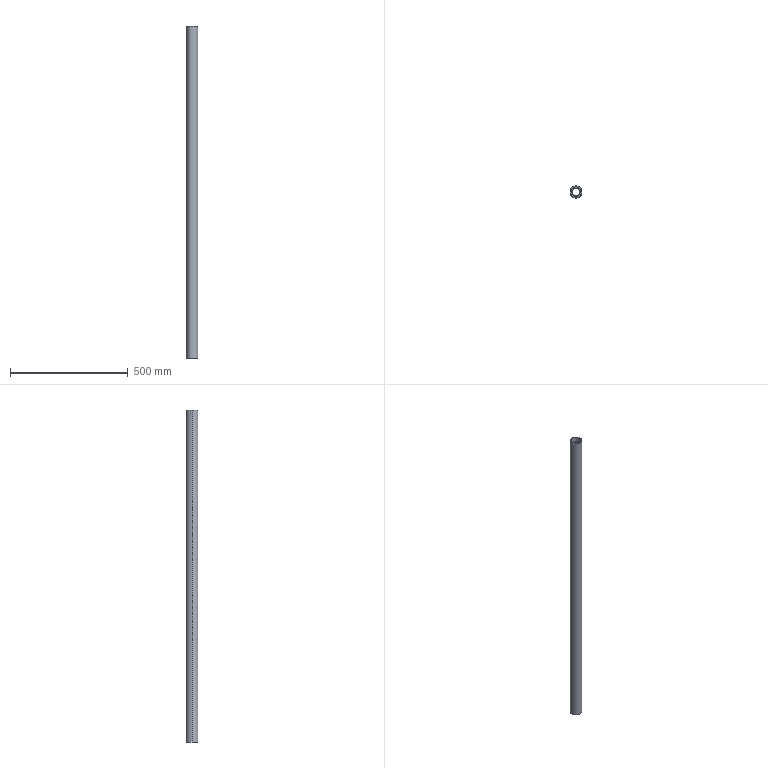Part | STEP file | 1 solid | 12 faces | box 50 x 50 x 1410 mm | volume 1744715 mm3 | cylinder 8 | plane 4 | commonest cylinder face diameters 42 x4 30 x2 50 x2
STEP:
#1=CARTESIAN_POINT('',(0.,0.,0.));
#2=DIRECTION('',(0.,0.,1.));
#3=DIRECTION('',(1.,0.,0.));
#4=AXIS2_PLACEMENT_3D('',#1,#2,#3);
#5=CARTESIAN_POINT('',(-21.,0.,-665.));
#6=VERTEX_POINT('',#5);
#7=CARTESIAN_POINT('',(-21.,0.,-685.));
#8=VERTEX_POINT('',#7);
#9=CARTESIAN_POINT('',(-21.,0.,-705.));
#10=DIRECTION('',(0.,0.,-1.));
#11=VECTOR('',#10,1.);
#12=LINE('',#9,#11);
#13=CARTESIAN_POINT('',(0.,0.,-705.));
#14=DIRECTION('',(0.,0.,-1.));
#15=DIRECTION('',(-1.,0.,0.));
#16=AXIS2_PLACEMENT_3D('',#13,#14,#15);
#17=CYLINDRICAL_SURFACE('',#16,21.);
#18=CARTESIAN_POINT('',(6.283,0.));
#19=DIRECTION('',(0.,1.));
#20=VECTOR('',#19,1.);
#21=LINE('',#18,#20);
#22=(GEOMETRIC_REPRESENTATION_CONTEXT(2)PARAMETRIC_REPRESENTATION_CONTEXT()REPRESENTATION_CONTEXT('',''));
#23=DEFINITIONAL_REPRESENTATION('',(#21),#22);
#24=PCURVE('',#17,#23);
#25=CARTESIAN_POINT('',(0.,0.,-705.));
#26=DIRECTION('',(0.,0.,-1.));
#27=DIRECTION('',(-1.,0.,0.));
#28=AXIS2_PLACEMENT_3D('',#25,#26,#27);
#29=CYLINDRICAL_SURFACE('',#28,21.);
#30=CARTESIAN_POINT('',(0.,0.));
#31=DIRECTION('',(0.,1.));
#32=VECTOR('',#31,1.);
#33=LINE('',#30,#32);
#34=(GEOMETRIC_REPRESENTATION_CONTEXT(2)PARAMETRIC_REPRESENTATION_CONTEXT()REPRESENTATION_CONTEXT('',''));
#35=DEFINITIONAL_REPRESENTATION('',(#33),#34);
#36=PCURVE('',#29,#35);
#37=SURFACE_CURVE('',#12,(#24,#36),.PCURVE_S1.);
#38=EDGE_CURVE('',#6,#8,#37,.T.);
#39=ORIENTED_EDGE('',*,*,#38,.T.);
#40=CARTESIAN_POINT('',(21.,0.,-685.));
#41=VERTEX_POINT('',#40);
#42=CARTESIAN_POINT('',(0.,0.,-685.));
#43=DIRECTION('',(0.,0.,1.));
#44=DIRECTION('',(1.,0.,0.));
#45=AXIS2_PLACEMENT_3D('',#42,#43,#44);
#46=CIRCLE('',#45,21.);
#47=CARTESIAN_POINT('',(9.425,-20.));
#48=DIRECTION('',(-1.,0.));
#49=VECTOR('',#48,1.);
#50=LINE('',#47,#49);
#51=(GEOMETRIC_REPRESENTATION_CONTEXT(2)PARAMETRIC_REPRESENTATION_CONTEXT()REPRESENTATION_CONTEXT('',''));
#52=DEFINITIONAL_REPRESENTATION('',(#50),#51);
#53=PCURVE('',#17,#52);
#54=CARTESIAN_POINT('',(0.,0.,-685.));
#55=DIRECTION('',(0.,0.,1.));
#56=DIRECTION('',(1.,0.,0.));
#57=AXIS2_PLACEMENT_3D('',#54,#55,#56);
#58=PLANE('',#57);
#59=CARTESIAN_POINT('',(0.,0.));
#60=DIRECTION('',(1.,0.));
#61=AXIS2_PLACEMENT_2D('',#59,#60);
#62=CIRCLE('',#61,21.);
#63=(GEOMETRIC_REPRESENTATION_CONTEXT(2)PARAMETRIC_REPRESENTATION_CONTEXT()REPRESENTATION_CONTEXT('',''));
#64=DEFINITIONAL_REPRESENTATION('',(#62),#63);
#65=PCURVE('',#58,#64);
#66=SURFACE_CURVE('',#46,(#53,#65),.PCURVE_S1.);
#67=EDGE_CURVE('',#8,#41,#66,.T.);
#68=ORIENTED_EDGE('',*,*,#67,.T.);
#69=CARTESIAN_POINT('',(21.,0.,-665.));
#70=VERTEX_POINT('',#69);
#71=CARTESIAN_POINT('',(21.,0.,-705.));
#72=DIRECTION('',(0.,0.,-1.));
#73=VECTOR('',#72,1.);
#74=LINE('',#71,#73);
#75=CARTESIAN_POINT('',(3.142,0.));
#76=DIRECTION('',(0.,1.));
#77=VECTOR('',#76,1.);
#78=LINE('',#75,#77);
#79=(GEOMETRIC_REPRESENTATION_CONTEXT(2)PARAMETRIC_REPRESENTATION_CONTEXT()REPRESENTATION_CONTEXT('',''));
#80=DEFINITIONAL_REPRESENTATION('',(#78),#79);
#81=PCURVE('',#17,#80);
#82=CARTESIAN_POINT('',(3.142,0.));
#83=DIRECTION('',(0.,1.));
#84=VECTOR('',#83,1.);
#85=LINE('',#82,#84);
#86=(GEOMETRIC_REPRESENTATION_CONTEXT(2)PARAMETRIC_REPRESENTATION_CONTEXT()REPRESENTATION_CONTEXT('',''));
#87=DEFINITIONAL_REPRESENTATION('',(#85),#86);
#88=PCURVE('',#29,#87);
#89=SURFACE_CURVE('',#74,(#81,#88),.PCURVE_S1.);
#90=EDGE_CURVE('',#70,#41,#89,.T.);
#91=ORIENTED_EDGE('',*,*,#90,.F.);
#92=CARTESIAN_POINT('',(0.,0.,-665.));
#93=DIRECTION('',(0.,0.,1.));
#94=DIRECTION('',(-1.,0.,0.));
#95=AXIS2_PLACEMENT_3D('',#92,#93,#94);
#96=CIRCLE('',#95,21.);
#97=CARTESIAN_POINT('',(6.283,-40.));
#98=DIRECTION('',(-1.,0.));
#99=VECTOR('',#98,1.);
#100=LINE('',#97,#99);
#101=(GEOMETRIC_REPRESENTATION_CONTEXT(2)PARAMETRIC_REPRESENTATION_CONTEXT()REPRESENTATION_CONTEXT('',''));
#102=DEFINITIONAL_REPRESENTATION('',(#100),#101);
#103=PCURVE('',#17,#102);
#104=CARTESIAN_POINT('',(0.,0.,-665.));
#105=DIRECTION('',(0.,0.,-1.));
#106=DIRECTION('',(1.,0.,0.));
#107=AXIS2_PLACEMENT_3D('',#104,#105,#106);
#108=PLANE('',#107);
#109=CARTESIAN_POINT('',(-21.,0.));
#110=CARTESIAN_POINT('',(-21.,36.373));
#111=CARTESIAN_POINT('',(10.5,18.187));
#112=CARTESIAN_POINT('',(42.,0.));
#113=CARTESIAN_POINT('',(10.5,-18.187));
#114=CARTESIAN_POINT('',(-21.,-36.373));
#115=CARTESIAN_POINT('',(-21.,0.));
#116=(BOUNDED_CURVE()B_SPLINE_CURVE(2,(#109,#110,#111,#112,#113,#114,#115),.UNSPECIFIED.,.T.,.F.)B_SPLINE_CURVE_WITH_KNOTS((1,2,2,2,2,1),(-2.094,0.,2.094,4.189,6.283,8.378),.UNSPECIFIED.)CURVE()GEOMETRIC_REPRESENTATION_ITEM()RATIONAL_B_SPLINE_CURVE((1.,0.5,1.,0.5,1.,0.5,1.))REPRESENTATION_ITEM(''));
#117=(GEOMETRIC_REPRESENTATION_CONTEXT(2)PARAMETRIC_REPRESENTATION_CONTEXT()REPRESENTATION_CONTEXT('',''));
#118=DEFINITIONAL_REPRESENTATION('',(#116),#117);
#119=PCURVE('',#108,#118);
#120=SURFACE_CURVE('',#96,(#103,#119),.PCURVE_S1.);
#121=EDGE_CURVE('',#6,#70,#120,.T.);
#122=ORIENTED_EDGE('',*,*,#121,.F.);
#123=EDGE_LOOP('',(#39,#68,#91,#122));
#124=FACE_BOUND('',#123,.F.);
#125=ADVANCED_FACE('',(#124),#17,.F.);
#126=CARTESIAN_POINT('',(21.,0.,705.));
#127=VERTEX_POINT('',#126);
#128=CARTESIAN_POINT('',(21.,0.,725.));
#129=VERTEX_POINT('',#128);
#130=CARTESIAN_POINT('',(21.,0.,705.));
#131=DIRECTION('',(0.,0.,1.));
#132=VECTOR('',#131,1.);
#133=LINE('',#130,#132);
#134=CARTESIAN_POINT('',(0.,0.,705.));
#135=DIRECTION('',(0.,0.,1.));
#136=DIRECTION('',(1.,0.,0.));
#137=AXIS2_PLACEMENT_3D('',#134,#135,#136);
#138=CYLINDRICAL_SURFACE('',#137,21.);
#139=CARTESIAN_POINT('',(6.283,0.));
#140=DIRECTION('',(0.,1.));
#141=VECTOR('',#140,1.);
#142=LINE('',#139,#141);
#143=(GEOMETRIC_REPRESENTATION_CONTEXT(2)PARAMETRIC_REPRESENTATION_CONTEXT()REPRESENTATION_CONTEXT('',''));
#144=DEFINITIONAL_REPRESENTATION('',(#142),#143);
#145=PCURVE('',#138,#144);
#146=CARTESIAN_POINT('',(0.,0.,705.));
#147=DIRECTION('',(0.,0.,1.));
#148=DIRECTION('',(1.,0.,0.));
#149=AXIS2_PLACEMENT_3D('',#146,#147,#148);
#150=CYLINDRICAL_SURFACE('',#149,21.);
#151=CARTESIAN_POINT('',(0.,0.));
#152=DIRECTION('',(0.,1.));
#153=VECTOR('',#152,1.);
#154=LINE('',#151,#153);
#155=(GEOMETRIC_REPRESENTATION_CONTEXT(2)PARAMETRIC_REPRESENTATION_CONTEXT()REPRESENTATION_CONTEXT('',''));
#156=DEFINITIONAL_REPRESENTATION('',(#154),#155);
#157=PCURVE('',#150,#156);
#158=SURFACE_CURVE('',#133,(#145,#157),.PCURVE_S1.);
#159=EDGE_CURVE('',#127,#129,#158,.T.);
#160=ORIENTED_EDGE('',*,*,#159,.T.);
#161=CARTESIAN_POINT('',(-21.,0.,725.));
#162=VERTEX_POINT('',#161);
#163=CARTESIAN_POINT('',(0.,0.,725.));
#164=DIRECTION('',(0.,0.,1.));
#165=DIRECTION('',(1.,0.,0.));
#166=AXIS2_PLACEMENT_3D('',#163,#164,#165);
#167=CIRCLE('',#166,21.);
#168=CARTESIAN_POINT('',(0.,20.));
#169=DIRECTION('',(1.,0.));
#170=VECTOR('',#169,1.);
#171=LINE('',#168,#170);
#172=(GEOMETRIC_REPRESENTATION_CONTEXT(2)PARAMETRIC_REPRESENTATION_CONTEXT()REPRESENTATION_CONTEXT('',''));
#173=DEFINITIONAL_REPRESENTATION('',(#171),#172);
#174=PCURVE('',#138,#173);
#175=CARTESIAN_POINT('',(0.,0.,725.));
#176=DIRECTION('',(0.,0.,1.));
#177=DIRECTION('',(1.,0.,0.));
#178=AXIS2_PLACEMENT_3D('',#175,#176,#177);
#179=PLANE('',#178);
#180=CARTESIAN_POINT('',(0.,0.));
#181=DIRECTION('',(1.,0.));
#182=AXIS2_PLACEMENT_2D('',#180,#181);
#183=CIRCLE('',#182,21.);
#184=(GEOMETRIC_REPRESENTATION_CONTEXT(2)PARAMETRIC_REPRESENTATION_CONTEXT()REPRESENTATION_CONTEXT('',''));
#185=DEFINITIONAL_REPRESENTATION('',(#183),#184);
#186=PCURVE('',#179,#185);
#187=SURFACE_CURVE('',#167,(#174,#186),.PCURVE_S1.);
#188=EDGE_CURVE('',#162,#129,#187,.T.);
#189=ORIENTED_EDGE('',*,*,#188,.F.);
#190=CARTESIAN_POINT('',(-21.,0.,705.));
#191=VERTEX_POINT('',#190);
#192=CARTESIAN_POINT('',(-21.,0.,705.));
#193=DIRECTION('',(0.,0.,1.));
#194=VECTOR('',#193,1.);
#195=LINE('',#192,#194);
#196=CARTESIAN_POINT('',(3.142,0.));
#197=DIRECTION('',(0.,1.));
#198=VECTOR('',#197,1.);
#199=LINE('',#196,#198);
#200=(GEOMETRIC_REPRESENTATION_CONTEXT(2)PARAMETRIC_REPRESENTATION_CONTEXT()REPRESENTATION_CONTEXT('',''));
#201=DEFINITIONAL_REPRESENTATION('',(#199),#200);
#202=PCURVE('',#138,#201);
#203=CARTESIAN_POINT('',(3.142,0.));
#204=DIRECTION('',(0.,1.));
#205=VECTOR('',#204,1.);
#206=LINE('',#203,#205);
#207=(GEOMETRIC_REPRESENTATION_CONTEXT(2)PARAMETRIC_REPRESENTATION_CONTEXT()REPRESENTATION_CONTEXT('',''));
#208=DEFINITIONAL_REPRESENTATION('',(#206),#207);
#209=PCURVE('',#150,#208);
#210=SURFACE_CURVE('',#195,(#202,#209),.PCURVE_S1.);
#211=EDGE_CURVE('',#191,#162,#210,.T.);
#212=ORIENTED_EDGE('',*,*,#211,.F.);
#213=CARTESIAN_POINT('',(0.,0.,705.));
#214=DIRECTION('',(0.,0.,1.));
#215=DIRECTION('',(1.,0.,0.));
#216=AXIS2_PLACEMENT_3D('',#213,#214,#215);
#217=CIRCLE('',#216,21.);
#218=CARTESIAN_POINT('',(0.,0.));
#219=DIRECTION('',(1.,0.));
#220=VECTOR('',#219,1.);
#221=LINE('',#218,#220);
#222=(GEOMETRIC_REPRESENTATION_CONTEXT(2)PARAMETRIC_REPRESENTATION_CONTEXT()REPRESENTATION_CONTEXT('',''));
#223=DEFINITIONAL_REPRESENTATION('',(#221),#222);
#224=PCURVE('',#138,#223);
#225=CARTESIAN_POINT('',(0.,0.,705.));
#226=DIRECTION('',(0.,0.,1.));
#227=DIRECTION('',(1.,0.,0.));
#228=AXIS2_PLACEMENT_3D('',#225,#226,#227);
#229=PLANE('',#228);
#230=CARTESIAN_POINT('',(0.,0.));
#231=DIRECTION('',(1.,0.));
#232=AXIS2_PLACEMENT_2D('',#230,#231);
#233=CIRCLE('',#232,21.);
#234=(GEOMETRIC_REPRESENTATION_CONTEXT(2)PARAMETRIC_REPRESENTATION_CONTEXT()REPRESENTATION_CONTEXT('',''));
#235=DEFINITIONAL_REPRESENTATION('',(#233),#234);
#236=PCURVE('',#229,#235);
#237=SURFACE_CURVE('',#217,(#224,#236),.PCURVE_S1.);
#238=EDGE_CURVE('',#191,#127,#237,.T.);
#239=ORIENTED_EDGE('',*,*,#238,.T.);
#240=EDGE_LOOP('',(#160,#189,#212,#239));
#241=FACE_BOUND('',#240,.F.);
#242=ADVANCED_FACE('',(#241),#138,.F.);
#243=CARTESIAN_POINT('',(25.,0.,725.));
#244=VERTEX_POINT('',#243);
#245=CARTESIAN_POINT('',(-25.,0.,725.));
#246=VERTEX_POINT('',#245);
#247=CARTESIAN_POINT('',(0.,0.,725.));
#248=DIRECTION('',(0.,0.,1.));
#249=DIRECTION('',(1.,0.,0.));
#250=AXIS2_PLACEMENT_3D('',#247,#248,#249);
#251=CIRCLE('',#250,25.);
#252=CARTESIAN_POINT('',(0.,0.,725.));
#253=DIRECTION('',(0.,0.,-1.));
#254=DIRECTION('',(-1.,0.,0.));
#255=AXIS2_PLACEMENT_3D('',#252,#253,#254);
#256=CYLINDRICAL_SURFACE('',#255,25.);
#257=CARTESIAN_POINT('',(3.142,0.));
#258=DIRECTION('',(-1.,0.));
#259=VECTOR('',#258,1.);
#260=LINE('',#257,#259);
#261=(GEOMETRIC_REPRESENTATION_CONTEXT(2)PARAMETRIC_REPRESENTATION_CONTEXT()REPRESENTATION_CONTEXT('',''));
#262=DEFINITIONAL_REPRESENTATION('',(#260),#261);
#263=PCURVE('',#256,#262);
#264=CARTESIAN_POINT('',(0.,0.));
#265=DIRECTION('',(1.,0.));
#266=AXIS2_PLACEMENT_2D('',#264,#265);
#267=CIRCLE('',#266,25.);
#268=(GEOMETRIC_REPRESENTATION_CONTEXT(2)PARAMETRIC_REPRESENTATION_CONTEXT()REPRESENTATION_CONTEXT('',''));
#269=DEFINITIONAL_REPRESENTATION('',(#267),#268);
#270=PCURVE('',#179,#269);
#271=SURFACE_CURVE('',#251,(#263,#270),.PCURVE_S1.);
#272=EDGE_CURVE('',#244,#246,#271,.T.);
#273=ORIENTED_EDGE('',*,*,#272,.F.);
#274=CARTESIAN_POINT('',(25.,0.,-685.));
#275=VERTEX_POINT('',#274);
#276=CARTESIAN_POINT('',(25.,0.,725.));
#277=DIRECTION('',(0.,0.,-1.));
#278=VECTOR('',#277,1.);
#279=LINE('',#276,#278);
#280=CARTESIAN_POINT('',(3.142,0.));
#281=DIRECTION('',(0.,1.));
#282=VECTOR('',#281,1.);
#283=LINE('',#280,#282);
#284=(GEOMETRIC_REPRESENTATION_CONTEXT(2)PARAMETRIC_REPRESENTATION_CONTEXT()REPRESENTATION_CONTEXT('',''));
#285=DEFINITIONAL_REPRESENTATION('',(#283),#284);
#286=PCURVE('',#256,#285);
#287=CARTESIAN_POINT('',(0.,0.,725.));
#288=DIRECTION('',(0.,0.,-1.));
#289=DIRECTION('',(-1.,0.,0.));
#290=AXIS2_PLACEMENT_3D('',#287,#288,#289);
#291=CYLINDRICAL_SURFACE('',#290,25.);
#292=CARTESIAN_POINT('',(3.142,0.));
#293=DIRECTION('',(0.,1.));
#294=VECTOR('',#293,1.);
#295=LINE('',#292,#294);
#296=(GEOMETRIC_REPRESENTATION_CONTEXT(2)PARAMETRIC_REPRESENTATION_CONTEXT()REPRESENTATION_CONTEXT('',''));
#297=DEFINITIONAL_REPRESENTATION('',(#295),#296);
#298=PCURVE('',#291,#297);
#299=SURFACE_CURVE('',#279,(#286,#298),.PCURVE_S1.);
#300=EDGE_CURVE('',#244,#275,#299,.T.);
#301=ORIENTED_EDGE('',*,*,#300,.T.);
#302=CARTESIAN_POINT('',(-25.,0.,-685.));
#303=VERTEX_POINT('',#302);
#304=CARTESIAN_POINT('',(0.,0.,-685.));
#305=DIRECTION('',(0.,0.,1.));
#306=DIRECTION('',(1.,0.,0.));
#307=AXIS2_PLACEMENT_3D('',#304,#305,#306);
#308=CIRCLE('',#307,25.);
#309=CARTESIAN_POINT('',(3.142,1410.));
#310=DIRECTION('',(-1.,0.));
#311=VECTOR('',#310,1.);
#312=LINE('',#309,#311);
#313=(GEOMETRIC_REPRESENTATION_CONTEXT(2)PARAMETRIC_REPRESENTATION_CONTEXT()REPRESENTATION_CONTEXT('',''));
#314=DEFINITIONAL_REPRESENTATION('',(#312),#313);
#315=PCURVE('',#256,#314);
#316=CARTESIAN_POINT('',(0.,0.));
#317=DIRECTION('',(1.,0.));
#318=AXIS2_PLACEMENT_2D('',#316,#317);
#319=CIRCLE('',#318,25.);
#320=(GEOMETRIC_REPRESENTATION_CONTEXT(2)PARAMETRIC_REPRESENTATION_CONTEXT()REPRESENTATION_CONTEXT('',''));
#321=DEFINITIONAL_REPRESENTATION('',(#319),#320);
#322=PCURVE('',#58,#321);
#323=SURFACE_CURVE('',#308,(#315,#322),.PCURVE_S1.);
#324=EDGE_CURVE('',#275,#303,#323,.T.);
#325=ORIENTED_EDGE('',*,*,#324,.T.);
#326=CARTESIAN_POINT('',(-25.,0.,725.));
#327=DIRECTION('',(0.,0.,-1.));
#328=VECTOR('',#327,1.);
#329=LINE('',#326,#328);
#330=CARTESIAN_POINT('',(0.,0.));
#331=DIRECTION('',(0.,1.));
#332=VECTOR('',#331,1.);
#333=LINE('',#330,#332);
#334=(GEOMETRIC_REPRESENTATION_CONTEXT(2)PARAMETRIC_REPRESENTATION_CONTEXT()REPRESENTATION_CONTEXT('',''));
#335=DEFINITIONAL_REPRESENTATION('',(#333),#334);
#336=PCURVE('',#256,#335);
#337=CARTESIAN_POINT('',(6.283,0.));
#338=DIRECTION('',(0.,1.));
#339=VECTOR('',#338,1.);
#340=LINE('',#337,#339);
#341=(GEOMETRIC_REPRESENTATION_CONTEXT(2)PARAMETRIC_REPRESENTATION_CONTEXT()REPRESENTATION_CONTEXT('',''));
#342=DEFINITIONAL_REPRESENTATION('',(#340),#341);
#343=PCURVE('',#291,#342);
#344=SURFACE_CURVE('',#329,(#336,#343),.PCURVE_S1.);
#345=EDGE_CURVE('',#246,#303,#344,.T.);
#346=ORIENTED_EDGE('',*,*,#345,.F.);
#347=EDGE_LOOP('',(#273,#301,#325,#346));
#348=FACE_BOUND('',#347,.T.);
#349=ADVANCED_FACE('',(#348),#256,.T.);
#350=CARTESIAN_POINT('',(-15.,0.,705.));
#351=VERTEX_POINT('',#350);
#352=CARTESIAN_POINT('',(-15.,0.,-665.));
#353=VERTEX_POINT('',#352);
#354=CARTESIAN_POINT('',(-15.,0.,725.));
#355=DIRECTION('',(0.,0.,-1.));
#356=VECTOR('',#355,1.);
#357=LINE('',#354,#356);
#358=CARTESIAN_POINT('',(0.,0.,725.));
#359=DIRECTION('',(0.,0.,-1.));
#360=DIRECTION('',(-1.,0.,0.));
#361=AXIS2_PLACEMENT_3D('',#358,#359,#360);
#362=CYLINDRICAL_SURFACE('',#361,15.);
#363=CARTESIAN_POINT('',(6.283,0.));
#364=DIRECTION('',(0.,1.));
#365=VECTOR('',#364,1.);
#366=LINE('',#363,#365);
#367=(GEOMETRIC_REPRESENTATION_CONTEXT(2)PARAMETRIC_REPRESENTATION_CONTEXT()REPRESENTATION_CONTEXT('',''));
#368=DEFINITIONAL_REPRESENTATION('',(#366),#367);
#369=PCURVE('',#362,#368);
#370=CARTESIAN_POINT('',(0.,0.,725.));
#371=DIRECTION('',(0.,0.,-1.));
#372=DIRECTION('',(-1.,0.,0.));
#373=AXIS2_PLACEMENT_3D('',#370,#371,#372);
#374=CYLINDRICAL_SURFACE('',#373,15.);
#375=CARTESIAN_POINT('',(0.,0.));
#376=DIRECTION('',(0.,1.));
#377=VECTOR('',#376,1.);
#378=LINE('',#375,#377);
#379=(GEOMETRIC_REPRESENTATION_CONTEXT(2)PARAMETRIC_REPRESENTATION_CONTEXT()REPRESENTATION_CONTEXT('',''));
#380=DEFINITIONAL_REPRESENTATION('',(#378),#379);
#381=PCURVE('',#374,#380);
#382=SURFACE_CURVE('',#357,(#369,#381),.PCURVE_S1.);
#383=EDGE_CURVE('',#351,#353,#382,.T.);
#384=ORIENTED_EDGE('',*,*,#383,.T.);
#385=CARTESIAN_POINT('',(15.,0.,-665.));
#386=VERTEX_POINT('',#385);
#387=CARTESIAN_POINT('',(0.,0.,-665.));
#388=DIRECTION('',(0.,0.,-1.));
#389=DIRECTION('',(-1.,0.,0.));
#390=AXIS2_PLACEMENT_3D('',#387,#388,#389);
#391=CIRCLE('',#390,15.);
#392=CARTESIAN_POINT('',(0.,1390.));
#393=DIRECTION('',(1.,0.));
#394=VECTOR('',#393,1.);
#395=LINE('',#392,#394);
#396=(GEOMETRIC_REPRESENTATION_CONTEXT(2)PARAMETRIC_REPRESENTATION_CONTEXT()REPRESENTATION_CONTEXT('',''));
#397=DEFINITIONAL_REPRESENTATION('',(#395),#396);
#398=PCURVE('',#362,#397);
#399=CARTESIAN_POINT('',(0.,0.));
#400=DIRECTION('',(-1.,0.));
#401=AXIS2_PLACEMENT_2D('',#399,#400);
#402=CIRCLE('',#401,15.);
#403=(GEOMETRIC_REPRESENTATION_CONTEXT(2)PARAMETRIC_REPRESENTATION_CONTEXT()REPRESENTATION_CONTEXT('',''));
#404=DEFINITIONAL_REPRESENTATION('',(#402),#403);
#405=PCURVE('',#108,#404);
#406=SURFACE_CURVE('',#391,(#398,#405),.PCURVE_S1.);
#407=EDGE_CURVE('',#386,#353,#406,.T.);
#408=ORIENTED_EDGE('',*,*,#407,.F.);
#409=CARTESIAN_POINT('',(15.,0.,705.));
#410=VERTEX_POINT('',#409);
#411=CARTESIAN_POINT('',(15.,0.,725.));
#412=DIRECTION('',(0.,0.,-1.));
#413=VECTOR('',#412,1.);
#414=LINE('',#411,#413);
#415=CARTESIAN_POINT('',(3.142,0.));
#416=DIRECTION('',(0.,1.));
#417=VECTOR('',#416,1.);
#418=LINE('',#415,#417);
#419=(GEOMETRIC_REPRESENTATION_CONTEXT(2)PARAMETRIC_REPRESENTATION_CONTEXT()REPRESENTATION_CONTEXT('',''));
#420=DEFINITIONAL_REPRESENTATION('',(#418),#419);
#421=PCURVE('',#362,#420);
#422=CARTESIAN_POINT('',(3.142,0.));
#423=DIRECTION('',(0.,1.));
#424=VECTOR('',#423,1.);
#425=LINE('',#422,#424);
#426=(GEOMETRIC_REPRESENTATION_CONTEXT(2)PARAMETRIC_REPRESENTATION_CONTEXT()REPRESENTATION_CONTEXT('',''));
#427=DEFINITIONAL_REPRESENTATION('',(#425),#426);
#428=PCURVE('',#374,#427);
#429=SURFACE_CURVE('',#414,(#421,#428),.PCURVE_S1.);
#430=EDGE_CURVE('',#410,#386,#429,.T.);
#431=ORIENTED_EDGE('',*,*,#430,.F.);
#432=CARTESIAN_POINT('',(0.,0.,705.));
#433=DIRECTION('',(0.,0.,1.));
#434=DIRECTION('',(1.,0.,0.));
#435=AXIS2_PLACEMENT_3D('',#432,#433,#434);
#436=CIRCLE('',#435,15.);
#437=CARTESIAN_POINT('',(9.425,20.));
#438=DIRECTION('',(-1.,0.));
#439=VECTOR('',#438,1.);
#440=LINE('',#437,#439);
#441=(GEOMETRIC_REPRESENTATION_CONTEXT(2)PARAMETRIC_REPRESENTATION_CONTEXT()REPRESENTATION_CONTEXT('',''));
#442=DEFINITIONAL_REPRESENTATION('',(#440),#441);
#443=PCURVE('',#362,#442);
#444=CARTESIAN_POINT('',(0.,0.));
#445=DIRECTION('',(1.,0.));
#446=AXIS2_PLACEMENT_2D('',#444,#445);
#447=CIRCLE('',#446,15.);
#448=(GEOMETRIC_REPRESENTATION_CONTEXT(2)PARAMETRIC_REPRESENTATION_CONTEXT()REPRESENTATION_CONTEXT('',''));
#449=DEFINITIONAL_REPRESENTATION('',(#447),#448);
#450=PCURVE('',#229,#449);
#451=SURFACE_CURVE('',#436,(#443,#450),.PCURVE_S1.);
#452=EDGE_CURVE('',#351,#410,#451,.T.);
#453=ORIENTED_EDGE('',*,*,#452,.F.);
#454=EDGE_LOOP('',(#384,#408,#431,#453));
#455=FACE_BOUND('',#454,.F.);
#456=ADVANCED_FACE('',(#455),#362,.F.);
#457=CARTESIAN_POINT('',(0.,0.,-665.));
#458=DIRECTION('',(0.,0.,-1.));
#459=DIRECTION('',(-1.,0.,0.));
#460=AXIS2_PLACEMENT_3D('',#457,#458,#459);
#461=CIRCLE('',#460,15.);
#462=CARTESIAN_POINT('',(0.,1390.));
#463=DIRECTION('',(1.,0.));
#464=VECTOR('',#463,1.);
#465=LINE('',#462,#464);
#466=(GEOMETRIC_REPRESENTATION_CONTEXT(2)PARAMETRIC_REPRESENTATION_CONTEXT()REPRESENTATION_CONTEXT('',''));
#467=DEFINITIONAL_REPRESENTATION('',(#465),#466);
#468=PCURVE('',#374,#467);
#469=CARTESIAN_POINT('',(0.,0.));
#470=DIRECTION('',(-1.,0.));
#471=AXIS2_PLACEMENT_2D('',#469,#470);
#472=CIRCLE('',#471,15.);
#473=(GEOMETRIC_REPRESENTATION_CONTEXT(2)PARAMETRIC_REPRESENTATION_CONTEXT()REPRESENTATION_CONTEXT('',''));
#474=DEFINITIONAL_REPRESENTATION('',(#472),#473);
#475=PCURVE('',#108,#474);
#476=SURFACE_CURVE('',#461,(#468,#475),.PCURVE_S1.);
#477=EDGE_CURVE('',#353,#386,#476,.T.);
#478=ORIENTED_EDGE('',*,*,#477,.F.);
#479=ORIENTED_EDGE('',*,*,#383,.F.);
#480=CARTESIAN_POINT('',(0.,0.,705.));
#481=DIRECTION('',(0.,0.,1.));
#482=DIRECTION('',(1.,0.,0.));
#483=AXIS2_PLACEMENT_3D('',#480,#481,#482);
#484=CIRCLE('',#483,15.);
#485=CARTESIAN_POINT('',(3.142,20.));
#486=DIRECTION('',(-1.,0.));
#487=VECTOR('',#486,1.);
#488=LINE('',#485,#487);
#489=(GEOMETRIC_REPRESENTATION_CONTEXT(2)PARAMETRIC_REPRESENTATION_CONTEXT()REPRESENTATION_CONTEXT('',''));
#490=DEFINITIONAL_REPRESENTATION('',(#488),#489);
#491=PCURVE('',#374,#490);
#492=CARTESIAN_POINT('',(0.,0.));
#493=DIRECTION('',(1.,0.));
#494=AXIS2_PLACEMENT_2D('',#492,#493);
#495=CIRCLE('',#494,15.);
#496=(GEOMETRIC_REPRESENTATION_CONTEXT(2)PARAMETRIC_REPRESENTATION_CONTEXT()REPRESENTATION_CONTEXT('',''));
#497=DEFINITIONAL_REPRESENTATION('',(#495),#496);
#498=PCURVE('',#229,#497);
#499=SURFACE_CURVE('',#484,(#491,#498),.PCURVE_S1.);
#500=EDGE_CURVE('',#410,#351,#499,.T.);
#501=ORIENTED_EDGE('',*,*,#500,.F.);
#502=ORIENTED_EDGE('',*,*,#430,.T.);
#503=EDGE_LOOP('',(#478,#479,#501,#502));
#504=FACE_BOUND('',#503,.F.);
#505=ADVANCED_FACE('',(#504),#374,.F.);
#506=ORIENTED_EDGE('',*,*,#300,.F.);
#507=CARTESIAN_POINT('',(0.,0.,725.));
#508=DIRECTION('',(0.,0.,1.));
#509=DIRECTION('',(1.,0.,0.));
#510=AXIS2_PLACEMENT_3D('',#507,#508,#509);
#511=CIRCLE('',#510,25.);
#512=CARTESIAN_POINT('',(9.425,0.));
#513=DIRECTION('',(-1.,0.));
#514=VECTOR('',#513,1.);
#515=LINE('',#512,#514);
#516=(GEOMETRIC_REPRESENTATION_CONTEXT(2)PARAMETRIC_REPRESENTATION_CONTEXT()REPRESENTATION_CONTEXT('',''));
#517=DEFINITIONAL_REPRESENTATION('',(#515),#516);
#518=PCURVE('',#291,#517);
#519=CARTESIAN_POINT('',(0.,0.));
#520=DIRECTION('',(1.,0.));
#521=AXIS2_PLACEMENT_2D('',#519,#520);
#522=CIRCLE('',#521,25.);
#523=(GEOMETRIC_REPRESENTATION_CONTEXT(2)PARAMETRIC_REPRESENTATION_CONTEXT()REPRESENTATION_CONTEXT('',''));
#524=DEFINITIONAL_REPRESENTATION('',(#522),#523);
#525=PCURVE('',#179,#524);
#526=SURFACE_CURVE('',#511,(#518,#525),.PCURVE_S1.);
#527=EDGE_CURVE('',#246,#244,#526,.T.);
#528=ORIENTED_EDGE('',*,*,#527,.F.);
#529=ORIENTED_EDGE('',*,*,#345,.T.);
#530=CARTESIAN_POINT('',(0.,0.,-685.));
#531=DIRECTION('',(0.,0.,1.));
#532=DIRECTION('',(1.,0.,0.));
#533=AXIS2_PLACEMENT_3D('',#530,#531,#532);
#534=CIRCLE('',#533,25.);
#535=CARTESIAN_POINT('',(9.425,1410.));
#536=DIRECTION('',(-1.,0.));
#537=VECTOR('',#536,1.);
#538=LINE('',#535,#537);
#539=(GEOMETRIC_REPRESENTATION_CONTEXT(2)PARAMETRIC_REPRESENTATION_CONTEXT()REPRESENTATION_CONTEXT('',''));
#540=DEFINITIONAL_REPRESENTATION('',(#538),#539);
#541=PCURVE('',#291,#540);
#542=CARTESIAN_POINT('',(0.,0.));
#543=DIRECTION('',(1.,0.));
#544=AXIS2_PLACEMENT_2D('',#542,#543);
#545=CIRCLE('',#544,25.);
#546=(GEOMETRIC_REPRESENTATION_CONTEXT(2)PARAMETRIC_REPRESENTATION_CONTEXT()REPRESENTATION_CONTEXT('',''));
#547=DEFINITIONAL_REPRESENTATION('',(#545),#546);
#548=PCURVE('',#58,#547);
#549=SURFACE_CURVE('',#534,(#541,#548),.PCURVE_S1.);
#550=EDGE_CURVE('',#303,#275,#549,.T.);
#551=ORIENTED_EDGE('',*,*,#550,.T.);
#552=EDGE_LOOP('',(#506,#528,#529,#551));
#553=FACE_BOUND('',#552,.T.);
#554=ADVANCED_FACE('',(#553),#291,.T.);
#555=CARTESIAN_POINT('',(0.,0.,725.));
#556=DIRECTION('',(0.,0.,1.));
#557=DIRECTION('',(1.,0.,0.));
#558=AXIS2_PLACEMENT_3D('',#555,#556,#557);
#559=CIRCLE('',#558,21.);
#560=CARTESIAN_POINT('',(0.,0.));
#561=DIRECTION('',(1.,0.));
#562=AXIS2_PLACEMENT_2D('',#560,#561);
#563=CIRCLE('',#562,21.);
#564=(GEOMETRIC_REPRESENTATION_CONTEXT(2)PARAMETRIC_REPRESENTATION_CONTEXT()REPRESENTATION_CONTEXT('',''));
#565=DEFINITIONAL_REPRESENTATION('',(#563),#564);
#566=PCURVE('',#179,#565);
#567=CARTESIAN_POINT('',(0.,20.));
#568=DIRECTION('',(1.,0.));
#569=VECTOR('',#568,1.);
#570=LINE('',#567,#569);
#571=(GEOMETRIC_REPRESENTATION_CONTEXT(2)PARAMETRIC_REPRESENTATION_CONTEXT()REPRESENTATION_CONTEXT('',''));
#572=DEFINITIONAL_REPRESENTATION('',(#570),#571);
#573=PCURVE('',#150,#572);
#574=SURFACE_CURVE('',#559,(#566,#573),.PCURVE_S1.);
#575=EDGE_CURVE('',#129,#162,#574,.T.);
#576=ORIENTED_EDGE('',*,*,#575,.F.);
#577=ORIENTED_EDGE('',*,*,#188,.F.);
#578=EDGE_LOOP('',(#576,#577));
#579=FACE_BOUND('',#578,.T.);
#580=ORIENTED_EDGE('',*,*,#527,.T.);
#581=ORIENTED_EDGE('',*,*,#272,.T.);
#582=EDGE_LOOP('',(#580,#581));
#583=FACE_BOUND('',#582,.T.);
#584=ADVANCED_FACE('',(#579,#583),#179,.T.);
#585=ORIENTED_EDGE('',*,*,#67,.T.);
#586=CARTESIAN_POINT('',(0.,0.,-685.));
#587=DIRECTION('',(0.,0.,1.));
#588=DIRECTION('',(1.,0.,0.));
#589=AXIS2_PLACEMENT_3D('',#586,#587,#588);
#590=CIRCLE('',#589,21.);
#591=CARTESIAN_POINT('',(0.,0.));
#592=DIRECTION('',(1.,0.));
#593=AXIS2_PLACEMENT_2D('',#591,#592);
#594=CIRCLE('',#593,21.);
#595=(GEOMETRIC_REPRESENTATION_CONTEXT(2)PARAMETRIC_REPRESENTATION_CONTEXT()REPRESENTATION_CONTEXT('',''));
#596=DEFINITIONAL_REPRESENTATION('',(#594),#595);
#597=PCURVE('',#58,#596);
#598=CARTESIAN_POINT('',(3.142,-20.));
#599=DIRECTION('',(-1.,0.));
#600=VECTOR('',#599,1.);
#601=LINE('',#598,#600);
#602=(GEOMETRIC_REPRESENTATION_CONTEXT(2)PARAMETRIC_REPRESENTATION_CONTEXT()REPRESENTATION_CONTEXT('',''));
#603=DEFINITIONAL_REPRESENTATION('',(#601),#602);
#604=PCURVE('',#29,#603);
#605=SURFACE_CURVE('',#590,(#597,#604),.PCURVE_S1.);
#606=EDGE_CURVE('',#41,#8,#605,.T.);
#607=ORIENTED_EDGE('',*,*,#606,.T.);
#608=EDGE_LOOP('',(#585,#607));
#609=FACE_BOUND('',#608,.T.);
#610=ORIENTED_EDGE('',*,*,#550,.F.);
#611=ORIENTED_EDGE('',*,*,#324,.F.);
#612=EDGE_LOOP('',(#610,#611));
#613=FACE_BOUND('',#612,.T.);
#614=ADVANCED_FACE('',(#609,#613),#58,.F.);
#615=ORIENTED_EDGE('',*,*,#575,.F.);
#616=ORIENTED_EDGE('',*,*,#159,.F.);
#617=CARTESIAN_POINT('',(0.,0.,705.));
#618=DIRECTION('',(0.,0.,1.));
#619=DIRECTION('',(1.,0.,0.));
#620=AXIS2_PLACEMENT_3D('',#617,#618,#619);
#621=CIRCLE('',#620,21.);
#622=CARTESIAN_POINT('',(0.,0.));
#623=DIRECTION('',(1.,0.));
#624=VECTOR('',#623,1.);
#625=LINE('',#622,#624);
#626=(GEOMETRIC_REPRESENTATION_CONTEXT(2)PARAMETRIC_REPRESENTATION_CONTEXT()REPRESENTATION_CONTEXT('',''));
#627=DEFINITIONAL_REPRESENTATION('',(#625),#626);
#628=PCURVE('',#150,#627);
#629=CARTESIAN_POINT('',(0.,0.));
#630=DIRECTION('',(1.,0.));
#631=AXIS2_PLACEMENT_2D('',#629,#630);
#632=CIRCLE('',#631,21.);
#633=(GEOMETRIC_REPRESENTATION_CONTEXT(2)PARAMETRIC_REPRESENTATION_CONTEXT()REPRESENTATION_CONTEXT('',''));
#634=DEFINITIONAL_REPRESENTATION('',(#632),#633);
#635=PCURVE('',#229,#634);
#636=SURFACE_CURVE('',#621,(#628,#635),.PCURVE_S1.);
#637=EDGE_CURVE('',#127,#191,#636,.T.);
#638=ORIENTED_EDGE('',*,*,#637,.T.);
#639=ORIENTED_EDGE('',*,*,#211,.T.);
#640=EDGE_LOOP('',(#615,#616,#638,#639));
#641=FACE_BOUND('',#640,.F.);
#642=ADVANCED_FACE('',(#641),#150,.F.);
#643=ORIENTED_EDGE('',*,*,#452,.F.);
#644=ORIENTED_EDGE('',*,*,#500,.F.);
#645=EDGE_LOOP('',(#643,#644));
#646=FACE_BOUND('',#645,.T.);
#647=ORIENTED_EDGE('',*,*,#637,.T.);
#648=ORIENTED_EDGE('',*,*,#238,.T.);
#649=EDGE_LOOP('',(#647,#648));
#650=FACE_BOUND('',#649,.T.);
#651=ADVANCED_FACE('',(#646,#650),#229,.T.);
#652=ORIENTED_EDGE('',*,*,#606,.T.);
#653=ORIENTED_EDGE('',*,*,#38,.F.);
#654=CARTESIAN_POINT('',(0.,0.,-665.));
#655=DIRECTION('',(0.,0.,1.));
#656=DIRECTION('',(-1.,0.,0.));
#657=AXIS2_PLACEMENT_3D('',#654,#655,#656);
#658=CIRCLE('',#657,21.);
#659=CARTESIAN_POINT('',(6.283,-40.));
#660=DIRECTION('',(-1.,0.));
#661=VECTOR('',#660,1.);
#662=LINE('',#659,#661);
#663=(GEOMETRIC_REPRESENTATION_CONTEXT(2)PARAMETRIC_REPRESENTATION_CONTEXT()REPRESENTATION_CONTEXT('',''));
#664=DEFINITIONAL_REPRESENTATION('',(#662),#663);
#665=PCURVE('',#29,#664);
#666=CARTESIAN_POINT('',(-21.,0.));
#667=CARTESIAN_POINT('',(-21.,36.373));
#668=CARTESIAN_POINT('',(10.5,18.187));
#669=CARTESIAN_POINT('',(42.,0.));
#670=CARTESIAN_POINT('',(10.5,-18.187));
#671=CARTESIAN_POINT('',(-21.,-36.373));
#672=CARTESIAN_POINT('',(-21.,0.));
#673=(BOUNDED_CURVE()B_SPLINE_CURVE(2,(#666,#667,#668,#669,#670,#671,#672),.UNSPECIFIED.,.T.,.F.)B_SPLINE_CURVE_WITH_KNOTS((1,2,2,2,2,1),(-2.094,0.,2.094,4.189,6.283,8.378),.UNSPECIFIED.)CURVE()GEOMETRIC_REPRESENTATION_ITEM()RATIONAL_B_SPLINE_CURVE((1.,0.5,1.,0.5,1.,0.5,1.))REPRESENTATION_ITEM(''));
#674=(GEOMETRIC_REPRESENTATION_CONTEXT(2)PARAMETRIC_REPRESENTATION_CONTEXT()REPRESENTATION_CONTEXT('',''));
#675=DEFINITIONAL_REPRESENTATION('',(#673),#674);
#676=PCURVE('',#108,#675);
#677=SURFACE_CURVE('',#658,(#665,#676),.PCURVE_S1.);
#678=EDGE_CURVE('',#70,#6,#677,.T.);
#679=ORIENTED_EDGE('',*,*,#678,.F.);
#680=ORIENTED_EDGE('',*,*,#90,.T.);
#681=EDGE_LOOP('',(#652,#653,#679,#680));
#682=FACE_BOUND('',#681,.F.);
#683=ADVANCED_FACE('',(#682),#29,.F.);
#684=ORIENTED_EDGE('',*,*,#477,.F.);
#685=ORIENTED_EDGE('',*,*,#407,.F.);
#686=EDGE_LOOP('',(#684,#685));
#687=FACE_BOUND('',#686,.T.);
#688=ORIENTED_EDGE('',*,*,#121,.F.);
#689=ORIENTED_EDGE('',*,*,#678,.F.);
#690=EDGE_LOOP('',(#688,#689));
#691=FACE_BOUND('',#690,.T.);
#692=ADVANCED_FACE('',(#687,#691),#108,.T.);
#693=CLOSED_SHELL('',(#125,#242,#349,#456,#505,#554,#584,#614,#642,#651,#683,#692));
#694=MANIFOLD_SOLID_BREP('',#693);
#695=(LENGTH_UNIT()NAMED_UNIT(*)SI_UNIT(.MILLI.,.METRE.));
#696=UNCERTAINTY_MEASURE_WITH_UNIT(LENGTH_MEASURE(0.0000001),#695,'','');
#697=(NAMED_UNIT(*)PLANE_ANGLE_UNIT()SI_UNIT($,.RADIAN.));
#698=(NAMED_UNIT(*)SI_UNIT($,.STERADIAN.)SOLID_ANGLE_UNIT());
#699=(GEOMETRIC_REPRESENTATION_CONTEXT(3)GLOBAL_UNCERTAINTY_ASSIGNED_CONTEXT((#696))GLOBAL_UNIT_ASSIGNED_CONTEXT((#695,#697,#698))REPRESENTATION_CONTEXT('',''));
#700=ADVANCED_BREP_SHAPE_REPRESENTATION('',(#4,#694),#699);